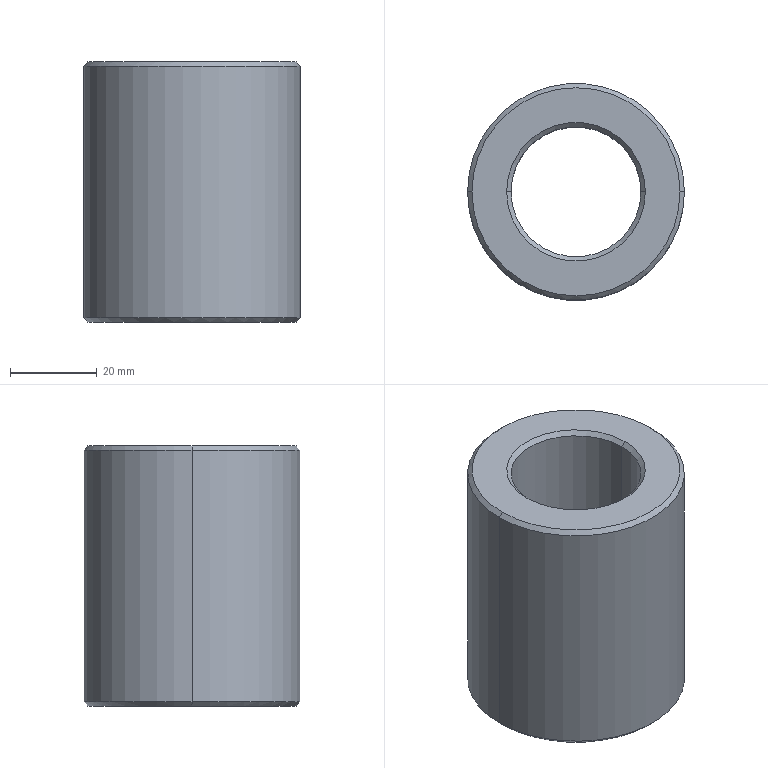Part | SolidWorks | features Chamfer 1, Extrusion 1 | 1 solid | 14 faces | box 50 x 50 x 60 mm | volume 75147 mm3 | cone 8 | cylinder 4 | plane 2 | commonest cylinder face diameters 30 x2 50 x2
STEP:
#1=CARTESIAN_POINT('',(24.,0.,60.));
#2=VERTEX_POINT('',#1);
#3=CARTESIAN_POINT('',(-24.,0.,60.));
#4=VERTEX_POINT('',#3);
#5=CARTESIAN_POINT('',(0.,0.,60.));
#6=DIRECTION('',(0.,0.,1.));
#7=DIRECTION('',(1.,0.,0.));
#8=AXIS2_PLACEMENT_3D('',#5,#6,#7);
#9=CIRCLE('',#8,24.);
#10=EDGE_CURVE('',#2,#4,#9,.T.);
#11=ORIENTED_EDGE('',*,*,#10,.F.);
#12=CARTESIAN_POINT('',(25.,0.,59.));
#13=VERTEX_POINT('',#12);
#14=CARTESIAN_POINT('',(24.,0.,60.));
#15=DIRECTION('',(0.7071,0.,-0.7071));
#16=VECTOR('',#15,1000.);
#17=LINE('',#14,#16);
#18=EDGE_CURVE('',#2,#13,#17,.T.);
#19=ORIENTED_EDGE('',*,*,#18,.T.);
#20=CARTESIAN_POINT('',(-25.,0.,59.));
#21=VERTEX_POINT('',#20);
#22=CARTESIAN_POINT('',(0.,0.,59.));
#23=DIRECTION('',(0.,0.,-1.));
#24=DIRECTION('',(1.,0.,0.));
#25=AXIS2_PLACEMENT_3D('',#22,#23,#24);
#26=CIRCLE('',#25,25.);
#27=EDGE_CURVE('',#21,#13,#26,.T.);
#28=ORIENTED_EDGE('',*,*,#27,.F.);
#29=CARTESIAN_POINT('',(-24.,0.,60.));
#30=DIRECTION('',(-0.7071,0.,-0.7071));
#31=VECTOR('',#30,1000.);
#32=LINE('',#29,#31);
#33=EDGE_CURVE('',#4,#21,#32,.T.);
#34=ORIENTED_EDGE('',*,*,#33,.F.);
#35=EDGE_LOOP('',(#11,#19,#28,#34));
#36=FACE_OUTER_BOUND('',#35,.T.);
#37=CARTESIAN_POINT('',(0.,0.,60.));
#38=DIRECTION('',(0.,0.,-1.));
#39=DIRECTION('',(-1.,0.,0.));
#40=AXIS2_PLACEMENT_3D('',#37,#38,#39);
#41=CONICAL_SURFACE('',#40,24.,0.7854);
#42=ADVANCED_FACE('',(#36),#41,.T.);
#43=CARTESIAN_POINT('',(-15.,0.,59.));
#44=VERTEX_POINT('',#43);
#45=CARTESIAN_POINT('',(15.,0.,59.));
#46=VERTEX_POINT('',#45);
#47=CARTESIAN_POINT('',(0.,0.,59.));
#48=DIRECTION('',(0.,0.,1.));
#49=DIRECTION('',(1.,0.,0.));
#50=AXIS2_PLACEMENT_3D('',#47,#48,#49);
#51=CIRCLE('',#50,15.);
#52=EDGE_CURVE('',#44,#46,#51,.T.);
#53=ORIENTED_EDGE('',*,*,#52,.F.);
#54=CARTESIAN_POINT('',(-16.,0.,60.));
#55=VERTEX_POINT('',#54);
#56=CARTESIAN_POINT('',(-15.,0.,59.));
#57=DIRECTION('',(-0.7071,0.,0.7071));
#58=VECTOR('',#57,1000.);
#59=LINE('',#56,#58);
#60=EDGE_CURVE('',#44,#55,#59,.T.);
#61=ORIENTED_EDGE('',*,*,#60,.T.);
#62=CARTESIAN_POINT('',(16.,0.,60.));
#63=VERTEX_POINT('',#62);
#64=CARTESIAN_POINT('',(0.,0.,60.));
#65=DIRECTION('',(0.,0.,-1.));
#66=DIRECTION('',(1.,0.,0.));
#67=AXIS2_PLACEMENT_3D('',#64,#65,#66);
#68=CIRCLE('',#67,16.);
#69=EDGE_CURVE('',#63,#55,#68,.T.);
#70=ORIENTED_EDGE('',*,*,#69,.F.);
#71=CARTESIAN_POINT('',(15.,0.,59.));
#72=DIRECTION('',(0.7071,0.,0.7071));
#73=VECTOR('',#72,1000.);
#74=LINE('',#71,#73);
#75=EDGE_CURVE('',#46,#63,#74,.T.);
#76=ORIENTED_EDGE('',*,*,#75,.F.);
#77=EDGE_LOOP('',(#53,#61,#70,#76));
#78=FACE_OUTER_BOUND('',#77,.T.);
#79=CARTESIAN_POINT('',(0.,0.,59.));
#80=DIRECTION('',(0.,0.,1.));
#81=DIRECTION('',(1.,0.,0.));
#82=AXIS2_PLACEMENT_3D('',#79,#80,#81);
#83=CONICAL_SURFACE('',#82,15.,0.7854);
#84=ADVANCED_FACE('',(#78),#83,.F.);
#85=CARTESIAN_POINT('',(-24.,0.,0.));
#86=VERTEX_POINT('',#85);
#87=CARTESIAN_POINT('',(24.,0.,0.));
#88=VERTEX_POINT('',#87);
#89=CARTESIAN_POINT('',(0.,0.,0.));
#90=DIRECTION('',(0.,0.,-1.));
#91=DIRECTION('',(1.,0.,0.));
#92=AXIS2_PLACEMENT_3D('',#89,#90,#91);
#93=CIRCLE('',#92,24.);
#94=EDGE_CURVE('',#86,#88,#93,.T.);
#95=ORIENTED_EDGE('',*,*,#94,.F.);
#96=CARTESIAN_POINT('',(-25.,0.,1.));
#97=VERTEX_POINT('',#96);
#98=CARTESIAN_POINT('',(-25.,0.,1.));
#99=DIRECTION('',(-0.7071,0.,0.7071));
#100=VECTOR('',#99,1000.);
#101=LINE('',#98,#100);
#102=EDGE_CURVE('',#86,#97,#101,.T.);
#103=ORIENTED_EDGE('',*,*,#102,.T.);
#104=CARTESIAN_POINT('',(25.,0.,1.));
#105=VERTEX_POINT('',#104);
#106=CARTESIAN_POINT('',(0.,0.,1.));
#107=DIRECTION('',(0.,0.,1.));
#108=DIRECTION('',(1.,0.,0.));
#109=AXIS2_PLACEMENT_3D('',#106,#107,#108);
#110=CIRCLE('',#109,25.);
#111=EDGE_CURVE('',#105,#97,#110,.T.);
#112=ORIENTED_EDGE('',*,*,#111,.F.);
#113=CARTESIAN_POINT('',(25.,0.,1.));
#114=DIRECTION('',(0.7071,0.,0.7071));
#115=VECTOR('',#114,1000.);
#116=LINE('',#113,#115);
#117=EDGE_CURVE('',#88,#105,#116,.T.);
#118=ORIENTED_EDGE('',*,*,#117,.F.);
#119=EDGE_LOOP('',(#95,#103,#112,#118));
#120=FACE_OUTER_BOUND('',#119,.T.);
#121=CARTESIAN_POINT('',(0.,0.,1.));
#122=DIRECTION('',(0.,0.,1.));
#123=DIRECTION('',(1.,0.,0.));
#124=AXIS2_PLACEMENT_3D('',#121,#122,#123);
#125=CONICAL_SURFACE('',#124,25.,0.7854);
#126=ADVANCED_FACE('',(#120),#125,.T.);
#127=CARTESIAN_POINT('',(15.,0.,1.));
#128=VERTEX_POINT('',#127);
#129=CARTESIAN_POINT('',(-15.,0.,1.));
#130=VERTEX_POINT('',#129);
#131=CARTESIAN_POINT('',(0.,0.,1.));
#132=DIRECTION('',(0.,0.,-1.));
#133=DIRECTION('',(1.,0.,0.));
#134=AXIS2_PLACEMENT_3D('',#131,#132,#133);
#135=CIRCLE('',#134,15.);
#136=EDGE_CURVE('',#128,#130,#135,.T.);
#137=ORIENTED_EDGE('',*,*,#136,.F.);
#138=CARTESIAN_POINT('',(16.,0.,0.));
#139=VERTEX_POINT('',#138);
#140=CARTESIAN_POINT('',(16.,0.,0.));
#141=DIRECTION('',(0.7071,0.,-0.7071));
#142=VECTOR('',#141,1000.);
#143=LINE('',#140,#142);
#144=EDGE_CURVE('',#128,#139,#143,.T.);
#145=ORIENTED_EDGE('',*,*,#144,.T.);
#146=CARTESIAN_POINT('',(-16.,0.,0.));
#147=VERTEX_POINT('',#146);
#148=CARTESIAN_POINT('',(0.,0.,0.));
#149=DIRECTION('',(0.,0.,1.));
#150=DIRECTION('',(1.,0.,0.));
#151=AXIS2_PLACEMENT_3D('',#148,#149,#150);
#152=CIRCLE('',#151,16.);
#153=EDGE_CURVE('',#147,#139,#152,.T.);
#154=ORIENTED_EDGE('',*,*,#153,.F.);
#155=CARTESIAN_POINT('',(-16.,0.,0.));
#156=DIRECTION('',(-0.7071,0.,-0.7071));
#157=VECTOR('',#156,1000.);
#158=LINE('',#155,#157);
#159=EDGE_CURVE('',#130,#147,#158,.T.);
#160=ORIENTED_EDGE('',*,*,#159,.F.);
#161=EDGE_LOOP('',(#137,#145,#154,#160));
#162=FACE_OUTER_BOUND('',#161,.T.);
#163=CARTESIAN_POINT('',(0.,0.,0.));
#164=DIRECTION('',(0.,0.,-1.));
#165=DIRECTION('',(-1.,0.,0.));
#166=AXIS2_PLACEMENT_3D('',#163,#164,#165);
#167=CONICAL_SURFACE('',#166,16.,0.7854);
#168=ADVANCED_FACE('',(#162),#167,.F.);
#169=ORIENTED_EDGE('',*,*,#52,.T.);
#170=CARTESIAN_POINT('',(15.,0.,60.));
#171=DIRECTION('',(0.,0.,-1.));
#172=VECTOR('',#171,1000.);
#173=LINE('',#170,#172);
#174=EDGE_CURVE('',#46,#128,#173,.T.);
#175=ORIENTED_EDGE('',*,*,#174,.T.);
#176=ORIENTED_EDGE('',*,*,#136,.T.);
#177=CARTESIAN_POINT('',(-15.,0.,60.));
#178=DIRECTION('',(0.,0.,-1.));
#179=VECTOR('',#178,1000.);
#180=LINE('',#177,#179);
#181=EDGE_CURVE('',#44,#130,#180,.T.);
#182=ORIENTED_EDGE('',*,*,#181,.F.);
#183=EDGE_LOOP('',(#169,#175,#176,#182));
#184=FACE_OUTER_BOUND('',#183,.T.);
#185=CARTESIAN_POINT('',(0.,0.,60.));
#186=DIRECTION('',(0.,0.,-1.));
#187=DIRECTION('',(-1.,0.,0.));
#188=AXIS2_PLACEMENT_3D('',#185,#186,#187);
#189=CYLINDRICAL_SURFACE('',#188,15.);
#190=ADVANCED_FACE('',(#184),#189,.F.);
#191=ORIENTED_EDGE('',*,*,#27,.T.);
#192=CARTESIAN_POINT('',(25.,0.,60.));
#193=DIRECTION('',(0.,0.,-1.));
#194=VECTOR('',#193,1000.);
#195=LINE('',#192,#194);
#196=EDGE_CURVE('',#13,#105,#195,.T.);
#197=ORIENTED_EDGE('',*,*,#196,.T.);
#198=ORIENTED_EDGE('',*,*,#111,.T.);
#199=CARTESIAN_POINT('',(-25.,0.,60.));
#200=DIRECTION('',(0.,0.,-1.));
#201=VECTOR('',#200,1000.);
#202=LINE('',#199,#201);
#203=EDGE_CURVE('',#21,#97,#202,.T.);
#204=ORIENTED_EDGE('',*,*,#203,.F.);
#205=EDGE_LOOP('',(#191,#197,#198,#204));
#206=FACE_OUTER_BOUND('',#205,.T.);
#207=CARTESIAN_POINT('',(0.,0.,60.));
#208=DIRECTION('',(0.,0.,-1.));
#209=DIRECTION('',(-1.,0.,0.));
#210=AXIS2_PLACEMENT_3D('',#207,#208,#209);
#211=CYLINDRICAL_SURFACE('',#210,25.);
#212=ADVANCED_FACE('',(#206),#211,.T.);
#213=ORIENTED_EDGE('',*,*,#69,.T.);
#214=CARTESIAN_POINT('',(0.,0.,60.));
#215=DIRECTION('',(0.,0.,-1.));
#216=DIRECTION('',(1.,0.,0.));
#217=AXIS2_PLACEMENT_3D('',#214,#215,#216);
#218=CIRCLE('',#217,16.);
#219=EDGE_CURVE('',#55,#63,#218,.T.);
#220=ORIENTED_EDGE('',*,*,#219,.T.);
#221=EDGE_LOOP('',(#213,#220));
#222=FACE_BOUND('',#221,.T.);
#223=CARTESIAN_POINT('',(0.,0.,60.));
#224=DIRECTION('',(0.,0.,1.));
#225=DIRECTION('',(1.,0.,0.));
#226=AXIS2_PLACEMENT_3D('',#223,#224,#225);
#227=CIRCLE('',#226,24.);
#228=EDGE_CURVE('',#4,#2,#227,.T.);
#229=ORIENTED_EDGE('',*,*,#228,.T.);
#230=ORIENTED_EDGE('',*,*,#10,.T.);
#231=EDGE_LOOP('',(#229,#230));
#232=FACE_OUTER_BOUND('',#231,.T.);
#233=CARTESIAN_POINT('',(0.,0.,60.));
#234=DIRECTION('',(0.,0.,1.));
#235=DIRECTION('',(1.,0.,0.));
#236=AXIS2_PLACEMENT_3D('',#233,#234,#235);
#237=PLANE('',#236);
#238=ADVANCED_FACE('',(#222,#232),#237,.T.);
#239=ORIENTED_EDGE('',*,*,#153,.T.);
#240=CARTESIAN_POINT('',(0.,0.,0.));
#241=DIRECTION('',(0.,0.,1.));
#242=DIRECTION('',(1.,0.,0.));
#243=AXIS2_PLACEMENT_3D('',#240,#241,#242);
#244=CIRCLE('',#243,16.);
#245=EDGE_CURVE('',#139,#147,#244,.T.);
#246=ORIENTED_EDGE('',*,*,#245,.T.);
#247=EDGE_LOOP('',(#239,#246));
#248=FACE_BOUND('',#247,.T.);
#249=CARTESIAN_POINT('',(0.,0.,0.));
#250=DIRECTION('',(0.,0.,-1.));
#251=DIRECTION('',(1.,0.,0.));
#252=AXIS2_PLACEMENT_3D('',#249,#250,#251);
#253=CIRCLE('',#252,24.);
#254=EDGE_CURVE('',#88,#86,#253,.T.);
#255=ORIENTED_EDGE('',*,*,#254,.T.);
#256=ORIENTED_EDGE('',*,*,#94,.T.);
#257=EDGE_LOOP('',(#255,#256));
#258=FACE_OUTER_BOUND('',#257,.T.);
#259=CARTESIAN_POINT('',(0.,0.,0.));
#260=DIRECTION('',(0.,0.,1.));
#261=DIRECTION('',(1.,0.,0.));
#262=AXIS2_PLACEMENT_3D('',#259,#260,#261);
#263=PLANE('',#262);
#264=ADVANCED_FACE('',(#248,#258),#263,.F.);
#265=ORIENTED_EDGE('',*,*,#196,.F.);
#266=CARTESIAN_POINT('',(0.,0.,59.));
#267=DIRECTION('',(0.,0.,-1.));
#268=DIRECTION('',(1.,0.,0.));
#269=AXIS2_PLACEMENT_3D('',#266,#267,#268);
#270=CIRCLE('',#269,25.);
#271=EDGE_CURVE('',#13,#21,#270,.T.);
#272=ORIENTED_EDGE('',*,*,#271,.T.);
#273=ORIENTED_EDGE('',*,*,#203,.T.);
#274=CARTESIAN_POINT('',(0.,0.,1.));
#275=DIRECTION('',(0.,0.,1.));
#276=DIRECTION('',(1.,0.,0.));
#277=AXIS2_PLACEMENT_3D('',#274,#275,#276);
#278=CIRCLE('',#277,25.);
#279=EDGE_CURVE('',#97,#105,#278,.T.);
#280=ORIENTED_EDGE('',*,*,#279,.T.);
#281=EDGE_LOOP('',(#265,#272,#273,#280));
#282=FACE_OUTER_BOUND('',#281,.T.);
#283=CARTESIAN_POINT('',(0.,0.,60.));
#284=DIRECTION('',(0.,0.,-1.));
#285=DIRECTION('',(-1.,0.,0.));
#286=AXIS2_PLACEMENT_3D('',#283,#284,#285);
#287=CYLINDRICAL_SURFACE('',#286,25.);
#288=ADVANCED_FACE('',(#282),#287,.T.);
#289=ORIENTED_EDGE('',*,*,#174,.F.);
#290=CARTESIAN_POINT('',(0.,0.,59.));
#291=DIRECTION('',(0.,0.,1.));
#292=DIRECTION('',(1.,0.,0.));
#293=AXIS2_PLACEMENT_3D('',#290,#291,#292);
#294=CIRCLE('',#293,15.);
#295=EDGE_CURVE('',#46,#44,#294,.T.);
#296=ORIENTED_EDGE('',*,*,#295,.T.);
#297=ORIENTED_EDGE('',*,*,#181,.T.);
#298=CARTESIAN_POINT('',(0.,0.,1.));
#299=DIRECTION('',(0.,0.,-1.));
#300=DIRECTION('',(1.,0.,0.));
#301=AXIS2_PLACEMENT_3D('',#298,#299,#300);
#302=CIRCLE('',#301,15.);
#303=EDGE_CURVE('',#130,#128,#302,.T.);
#304=ORIENTED_EDGE('',*,*,#303,.T.);
#305=EDGE_LOOP('',(#289,#296,#297,#304));
#306=FACE_OUTER_BOUND('',#305,.T.);
#307=CARTESIAN_POINT('',(0.,0.,60.));
#308=DIRECTION('',(0.,0.,-1.));
#309=DIRECTION('',(-1.,0.,0.));
#310=AXIS2_PLACEMENT_3D('',#307,#308,#309);
#311=CYLINDRICAL_SURFACE('',#310,15.);
#312=ADVANCED_FACE('',(#306),#311,.F.);
#313=ORIENTED_EDGE('',*,*,#144,.F.);
#314=ORIENTED_EDGE('',*,*,#303,.F.);
#315=ORIENTED_EDGE('',*,*,#159,.T.);
#316=ORIENTED_EDGE('',*,*,#245,.F.);
#317=EDGE_LOOP('',(#313,#314,#315,#316));
#318=FACE_OUTER_BOUND('',#317,.T.);
#319=CARTESIAN_POINT('',(0.,0.,0.));
#320=DIRECTION('',(0.,0.,-1.));
#321=DIRECTION('',(-1.,0.,0.));
#322=AXIS2_PLACEMENT_3D('',#319,#320,#321);
#323=CONICAL_SURFACE('',#322,16.,0.7854);
#324=ADVANCED_FACE('',(#318),#323,.F.);
#325=ORIENTED_EDGE('',*,*,#102,.F.);
#326=ORIENTED_EDGE('',*,*,#254,.F.);
#327=ORIENTED_EDGE('',*,*,#117,.T.);
#328=ORIENTED_EDGE('',*,*,#279,.F.);
#329=EDGE_LOOP('',(#325,#326,#327,#328));
#330=FACE_OUTER_BOUND('',#329,.T.);
#331=CARTESIAN_POINT('',(0.,0.,1.));
#332=DIRECTION('',(0.,0.,1.));
#333=DIRECTION('',(1.,0.,0.));
#334=AXIS2_PLACEMENT_3D('',#331,#332,#333);
#335=CONICAL_SURFACE('',#334,25.,0.7854);
#336=ADVANCED_FACE('',(#330),#335,.T.);
#337=ORIENTED_EDGE('',*,*,#60,.F.);
#338=ORIENTED_EDGE('',*,*,#295,.F.);
#339=ORIENTED_EDGE('',*,*,#75,.T.);
#340=ORIENTED_EDGE('',*,*,#219,.F.);
#341=EDGE_LOOP('',(#337,#338,#339,#340));
#342=FACE_OUTER_BOUND('',#341,.T.);
#343=CARTESIAN_POINT('',(0.,0.,59.));
#344=DIRECTION('',(0.,0.,1.));
#345=DIRECTION('',(1.,0.,0.));
#346=AXIS2_PLACEMENT_3D('',#343,#344,#345);
#347=CONICAL_SURFACE('',#346,15.,0.7854);
#348=ADVANCED_FACE('',(#342),#347,.F.);
#349=ORIENTED_EDGE('',*,*,#18,.F.);
#350=ORIENTED_EDGE('',*,*,#228,.F.);
#351=ORIENTED_EDGE('',*,*,#33,.T.);
#352=ORIENTED_EDGE('',*,*,#271,.F.);
#353=EDGE_LOOP('',(#349,#350,#351,#352));
#354=FACE_OUTER_BOUND('',#353,.T.);
#355=CARTESIAN_POINT('',(0.,0.,60.));
#356=DIRECTION('',(0.,0.,-1.));
#357=DIRECTION('',(-1.,0.,0.));
#358=AXIS2_PLACEMENT_3D('',#355,#356,#357);
#359=CONICAL_SURFACE('',#358,24.,0.7854);
#360=ADVANCED_FACE('',(#354),#359,.T.);
#361=CLOSED_SHELL('',(#42,#84,#126,#168,#190,#212,#238,#264,#288,#312,#324,#336,#348,#360));
#362=MANIFOLD_SOLID_BREP('',#361);
#363=CARTESIAN_POINT('',(0.,0.,0.));
#364=DIRECTION('',(0.,0.,1.));
#365=DIRECTION('',(1.,0.,0.));
#366=AXIS2_PLACEMENT_3D('',#363,#364,#365);
#367=(LENGTH_UNIT()NAMED_UNIT(*)SI_UNIT(.MILLI.,.METRE.));
#368=UNCERTAINTY_MEASURE_WITH_UNIT(LENGTH_MEASURE(0.00001),#367,'','');
#369=(NAMED_UNIT(*)PLANE_ANGLE_UNIT()SI_UNIT($,.RADIAN.));
#370=(NAMED_UNIT(*)SI_UNIT($,.STERADIAN.)SOLID_ANGLE_UNIT());
#371=(GEOMETRIC_REPRESENTATION_CONTEXT(3)GLOBAL_UNCERTAINTY_ASSIGNED_CONTEXT((#368))GLOBAL_UNIT_ASSIGNED_CONTEXT((#367,#369,#370))REPRESENTATION_CONTEXT('',''));
#372=ADVANCED_BREP_SHAPE_REPRESENTATION('',(#362,#366),#371);